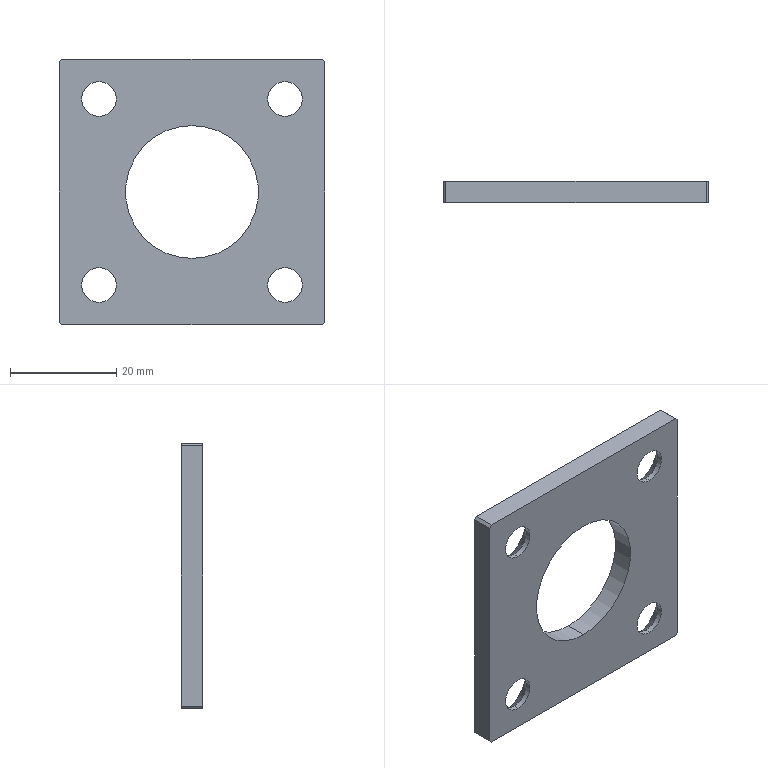Part | STEP file | Cuon T phu H01_4 | 1 solid | 28 faces | box 50 x 4 x 50 mm | volume 7023 mm3 | cylinder 10 | plane 10 | cone 8 | commonest cylinder face diameters 6.5 x8 25 x2